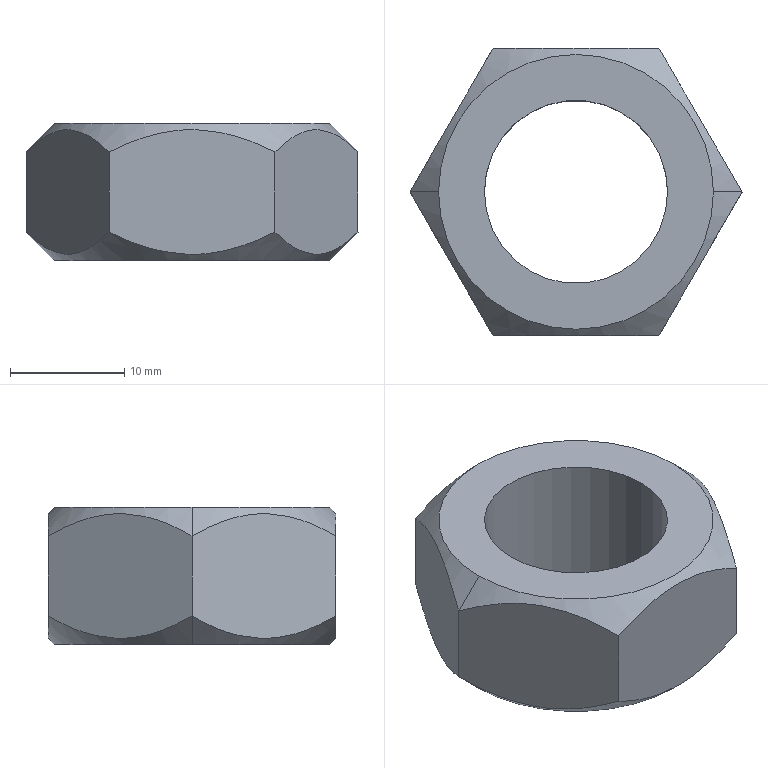Part | Creo | features DATUM PLANE 3, CURVE 2, CHAMFER 1, COORDINATE SYSTEM 1, CUT 1, PROTRUSION 1 | 1 solid | 14 faces | volume 4002 mm3 | plane 8 | cone 4 | cylinder 2 | commonest cylinder face diameters 16 x2